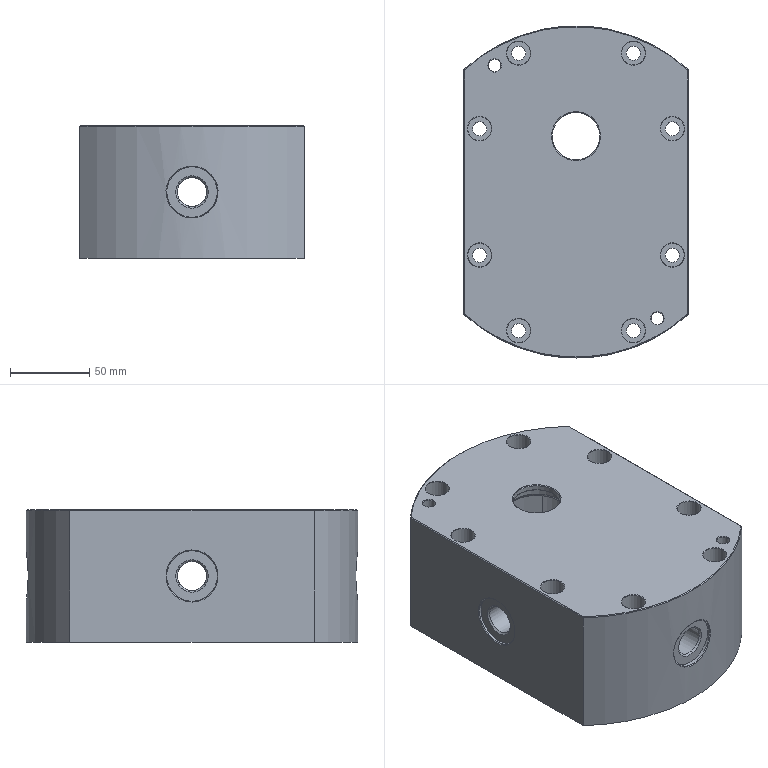NC program | NX | posted with a generic post | part box 142 x 210 x 84 mm
Whole program:
N10 G17 G21 G94 G90
(FLOOR_WALL , TOOL : D50)
N12 T02 M6
N14 G54
N16 G17 G0 G90 X46.563 Y-51.997 B0. C0. S1200 M3
N18 G43 Z30. H2
N20 Z2.65
N22 G94 G1 Z-0.35 F1000.
N24 X43.563
N26 X-43.563 F2000.
N28 Y-23.998
N30 X43.563
N32 Y4.001
N34 X-43.563
N36 Y32.
N38 X43.563
N40 X46.563
N42 Z2.65
N44 G0 Z30.
N46 X50.098 Y-51.997
N48 Z2.301
N50 G1 Z-0.699 F1000.
N52 X47.098
N54 X-47.098 F2000.
N56 Y-23.998
N58 X47.098
N60 Y4.001
N62 X-47.098
N64 Y32.
N66 X47.098
N68 X50.098
N70 Z2.301
N72 G0 Z30.
N74 X52.803 Y-51.997
N76 Z1.951
N78 G1 Z-1.049 F1000.
N80 X49.803
N82 X-49.803 F2000.
N84 Y-23.998
N86 X49.803
N88 Y4.001
N90 X-49.803
N92 Y32.
N94 X49.803
N96 X52.803
N98 Z1.951
N100 G0 Z30.
N102 X55.078 Y-51.997
N104 Z1.602
N106 G1 Z-1.398 F1000.
N108 X52.078
N110 X-52.078 F2000.
N112 Y-23.998
N114 X52.078
N116 Y4.001
N118 X-52.078
N120 Y32.
N122 X52.078
N124 X55.078
N126 Z1.602
N128 G0 Z30.
N130 X57.078 Y-51.997
N132 Z1.252
N134 G1 Z-1.748 F1000.
N136 X54.078
N138 X-54.078 F2000.
N140 Y-23.998
N142 X54.078
N144 Y4.001
N146 X-54.078
N148 Y32.
N150 X54.078
N152 X57.078
N154 Z1.252
N156 G0 Z30.
N158 X58.881 Y-51.997
N160 Z0.903
N162 G1 Z-2.097 F1000.
N164 X55.881
N166 X-55.881 F2000.
N168 Y-23.998
N170 X55.881
N172 Y4.001
N174 X-55.881
N176 Y32.
N178 X55.881
N180 X58.881
N182 Z0.903
N184 G0 Z30.
N186 X60.535 Y-51.997
N188 Z0.553
N190 G1 Z-2.447 F1000.
N192 X57.535
N194 X-57.535 F2000.
N196 Y-23.998
N198 X57.535
N200 Y4.001
N202 X-57.535
N204 Y32.
N206 X57.535
N208 X60.535
N210 Z0.553
N212 G0 Z30.
N214 X62.07 Y-51.997
N216 Z0.204
N218 G1 Z-2.796 F1000.
N220 X59.07
N222 X-59.07 F2000.
N224 Y-23.998
N226 X59.07
N228 Y4.001
N230 X-59.07
N232 Y32.
N234 X59.07
N236 X62.07
N238 Z0.204
N240 G0 Z30.
N242 X63.509 Y-51.997
N244 Z-0.146
N246 G1 Z-3.146 F1000.
N248 X60.509
N250 X-60.509 F2000.
N252 Y-23.998
N254 X60.509
N256 Y4.001
N258 X-60.509
N260 Y32.
N262 X60.509
N264 X63.509
N266 Z-0.146
N268 G0 Z30.
N270 X64.866 Y-51.997
N272 Z-0.495
N274 G1 Z-3.495 F1000.
N276 X61.866
N278 X-61.866 F2000.
N280 Y-23.998
N282 X61.866
N284 Y4.001
N286 X-61.866
N288 Y32.
N290 X61.866
N292 X64.866
N294 Z-0.495
N296 G0 Z30.
N298 X66.153 Y-51.997
N300 Z-0.845
N302 G1 Z-3.845 F1000.
N304 X63.153
N306 X-63.153 F2000.
N308 Y-23.998
N310 X63.153
N312 Y4.001
N314 X-63.153
N316 Y32.
N318 X63.153
N320 X66.153
N322 Z-0.845
N324 G0 Z30.
N326 X67.38 Y-51.997
N328 Z-1.194
N330 G1 Z-4.194 F1000.
N332 X64.38
N334 X-64.38 F2000.
N336 Y-23.998
N338 X64.38
N340 Y4.001
N342 X-64.38
N344 Y32.
N346 X64.38
N348 X67.38
N350 Z-1.194
N352 G0 Z30.
N354 X68.553 Y-51.997
N356 Z-1.544
N358 G1 Z-4.544 F1000.
N360 X65.553
N362 X-65.553 F2000.
N364 Y-23.998
N366 X65.553
N368 Y4.001
N370 X-65.553
N372 Y32.
N374 X65.553
N376 X68.553
N378 Z-1.544
N380 G0 Z30.
N382 X69.68 Y-51.997
N384 Z-1.893
N386 G1 Z-4.893 F1000.
N388 X66.68
N390 X-66.68 F2000.
N392 Y-23.998
N394 X66.68
N396 Y4.001
N398 X-66.68
N400 Y32.
N402 X66.68
N404 X69.68
N406 Z-1.893
N408 G0 Z30.
N410 X70.763 Y-51.997
N412 Z-2.243
N414 G1 Z-5.243 F1000.
N416 X67.763
N418 X-67.763 F2000.
N420 Y-23.998
N422 X67.763
N424 Y4.001
N426 X-67.763
N428 Y32.
N430 X67.763
N432 X70.763
N434 Z-2.243
N436 G0 Z30.
N438 X71.809 Y-51.997
N440 Z-2.592
N442 G1 Z-5.592 F1000.
N444 X68.809
N446 X-68.809 F2000.
N448 Y-23.998
N450 X68.809
N452 Y4.001
N454 X-68.809
N456 Y32.
N458 X68.809
N460 X71.809
N462 Z-2.592
N464 G0 Z30.
N466 X72.82 Y-51.997
N468 Z-2.941
N470 G1 Z-5.941 F1000.
N472 X69.82
N474 X-69.82 F2000.
N476 Y-23.998
N478 X69.82
N480 Y4.001
N482 X-69.82
N484 Y32.
N486 X69.82
N488 X72.82
N490 Z-2.941
N492 G0 Z30.
N494 X73.798 Y-51.997
N496 Z-3.291
N498 G1 Z-6.291 F1000.
N500 X70.798
N502 X-70.798 F2000.
N504 Y-23.998
N506 X70.798
N508 Y4.001
N510 X-70.798
N512 Y32.
N514 X70.798
N516 X73.798
N518 Z-3.291
N520 G0 Z30.
N522 X74.748 Y-51.997
N524 Z-3.64
N526 G1 Z-6.64 F1000.
N528 X71.748
N530 X-71.748 F2000.
N532 Y-23.998
N534 X71.748
N536 Y4.001
N538 X-71.748
N540 Y32.
N542 X71.748
N544 X74.748
N546 Z-3.64
N548 G0 Z30.
N550 X75.67 Y-51.997
N552 Z-3.99
N554 G1 Z-6.99 F1000.
N556 X72.67
N558 X-72.67 F2000.
N560 Y-23.998
N562 X72.67
N564 Y4.001
N566 X-72.67
N568 Y32.
N570 X72.67
N572 X75.67
N574 Z-3.99
N576 G0 Z30.
N578 X76.567 Y-51.997
N580 Z-4.339
N582 G1 Z-7.339 F1000.
N584 X73.567
N586 X-73.567 F2000.
N588 Y-23.998
N590 X73.567
N592 Y4.001
N594 X-73.567
N596 Y32.
N598 X73.567
N600 X76.567
N602 Z-4.339
N604 G0 Z30.
N606 X77.44 Y-51.997
N608 Z-4.689
N610 G1 Z-7.689 F1000.
N612 X74.44
N614 X-74.44 F2000.
N616 Y-23.998
N618 X74.44
N620 Y4.001
N622 X-74.44
N624 Y32.
N626 X74.44
N628 X77.44
N630 Z-4.689
N632 G0 Z30.
N634 X78.292 Y-51.997
N636 Z-5.038
N638 G1 Z-8.038 F1000.
N640 X75.292
N642 X-75.292 F2000.
N644 Y-23.998
N646 X75.292
N648 Y4.001
N650 X-75.292
N652 Y32.
N654 X75.292
N656 X78.292
N658 Z-5.038
N660 G0 Z30.
N662 X79.123 Y-51.997
N664 Z-5.388
N666 G1 Z-8.388 F1000.
N668 X76.123
N670 X-76.123 F2000.
N672 Y-23.998
N674 X76.123
N676 Y4.001
N678 X-76.123
N680 Y32.
N682 X76.123
N684 X79.123
N686 Z-5.388
N688 G0 Z30.
N690 X79.934 Y-51.997
N692 Z-5.737
N694 G1 Z-8.737 F1000.
N696 X76.934
N698 X-76.934 F2000.
N700 Y-23.998
N702 X76.934
N704 Y4.001
N706 X-76.934
N708 Y32.
N710 X76.934
N712 X79.934
N714 Z-5.737
N716 G0 Z30.
N718 X80.728 Y-51.997
N720 Z-6.087
N722 G1 Z-9.087 F1000.
N724 X77.728
N726 X-77.728 F2000.
N728 Y-23.998
N730 X77.728
N732 Y4.001
N734 X-77.728
N736 Y32.
N738 X77.728
N740 X80.728
N742 Z-6.087
N744 G0 Z30.
N746 X81.504 Y-51.997
N748 Z-6.436
N750 G1 Z-9.436 F1000.
N752 X78.504
N754 X-78.504 F2000.
N756 Y-23.998
N758 X78.504
N760 Y4.001
N762 X-78.504
N764 Y32.
N766 X78.504
N768 X81.504
N770 Z-6.436
N772 G0 Z30.
N774 X82.263 Y-51.997
N776 Z-6.786
N778 G1 Z-9.786 F1000.
N780 X79.263
N782 X-79.263 F2000.
N784 Y-23.998
N786 X79.263
N788 Y4.001
N790 X-79.263
N792 Y32.
N794 X79.263
N796 X82.263
N798 Z-6.786
N800 G0 Z30.
N802 X83.008 Y-51.997
N804 Z-7.135
N806 G1 Z-10.135 F1000.
N808 X80.008
N810 X-80.008 F2000.
N812 Y-23.998
N814 X80.008
N816 Y4.001
N818 X-80.008
N820 Y32.
N822 X80.008
N824 X83.008
N826 Z-7.135
N828 G0 Z30.
N830 X83.737 Y-51.997
N832 Z-7.485
N834 G1 Z-10.485 F1000.
N836 X80.737
N838 X-80.737 F2000.
N840 Y-23.998
N842 X80.737
N844 Y4.001
N846 X-80.737
N848 Y32.
N850 X80.737
N852 X83.737
N854 Z-7.485
N856 G0 Z30.
N858 X84.452 Y-51.997
N860 Z-7.834
N862 G1 Z-10.834 F1000.
N864 X81.452
N866 X-81.452 F2000.
N868 Y-23.998
N870 X81.452
N872 Y4.001
N874 X-81.452
N876 Y32.
N878 X81.452
N880 X84.452
N882 Z-7.834
N884 G0 Z30.
N886 X85.154 Y-51.997
N888 Z-8.184
N890 G1 Z-11.184 F1000.
N892 X82.154
N894 X-82.154 F2000.
N896 Y-23.998
N898 X82.154
N900 Y4.001
N902 X-82.154
N904 Y32.
N906 X82.154
N908 X85.154
N910 Z-8.184
N912 G0 Z30.
N914 X85.843 Y-51.997
N916 Z-8.533
N918 G1 Z-11.533 F1000.
N920 X82.843
N922 X-82.843 F2000.
N924 Y-23.998
N926 X82.843
N928 Y4.001
N930 X-82.843
N932 Y32.
N934 X82.843
N936 X85.843
N938 Z-8.533
N940 G0 Z30.
N942 X86.52 Y-51.997
N944 Z-8.883
N946 G1 Z-11.883 F1000.
N948 X83.52
N950 X-83.52 F2000.
N952 Y-23.998
N954 X83.52
N956 Y4.001
N958 X-83.52
N960 Y32.
N962 X83.52
N964 X86.52
N966 Z-8.883
N968 G0 Z30.
N970 X87.185 Y-51.997
N972 Z-9.232
N974 G1 Z-12.232 F1000.
N976 X84.185
N978 X-84.185 F2000.
N980 Y-23.998
N982 X84.185
N984 Y4.001
N986 X-84.185
N988 Y32.
N990 X84.185
N992 X87.185
N994 Z-9.232
N996 G0 Z30.
N998 X87.838 Y-51.997
N1000 Z-9.582
N1002 G1 Z-12.582 F1000.
N1004 X84.838
N1006 X-84.838 F2000.
N1008 Y-23.998
N1010 X84.838
N1012 Y4.001
N1014 X-84.838
N1016 Y32.
N1018 X84.838
N1020 X87.838
N1022 Z-9.582
N1024 G0 Z30.
N1026 X88.481 Y-51.997
N1028 Z-9.931
N1030 G1 Z-12.931 F1000.
N1032 X85.481
N1034 X-85.481 F2000.
N1036 Y-23.998
N1038 X85.481
N1040 Y4.001
N1042 X-85.481
N1044 Y32.
N1046 X85.481
N1048 X88.481
N1050 Z-9.931
N1052 G0 Z30.
N1054 X89.113 Y-51.997
N1056 Z-10.281
N1058 G1 Z-13.281 F1000.
N1060 X86.113
N1062 X-86.113 F2000.
N1064 Y-23.998
N1066 X86.113
N1068 Y4.001
N1070 X-86.113
N1072 Y32.
N1074 X86.113
N1076 X89.113
N1078 Z-10.281
N1080 G0 Z30.
N1082 X89.735 Y-51.997
N1084 Z-10.63
N1086 G1 Z-13.63 F1000.
N1088 X86.735
N1090 X-86.735 F2000.
N1092 Y-23.998
N1094 X86.735
N1096 Y4.001
N1098 X-86.735
N1100 Y32.
N1102 X86.735
N1104 X89.735
N1106 Z-10.63
N1108 G0 Z30.
N1110 X90.348 Y-51.997
N1112 Z-10.98
N1114 G1 Z-13.98 F1000.
N1116 X87.348
N1118 X-87.348 F2000.
N1120 Y-23.998
N1122 X87.348
N1124 Y4.001
N1126 X-87.348
N1128 Y32.
N1130 X87.348
N1132 X90.348
N1134 Z-10.98
N1136 G0 Z30.
N1138 X90.951 Y-51.997
N1140 Z-11.329
N1142 G1 Z-14.329 F1000.
N1144 X87.951
N1146 X-87.951 F2000.
N1148 Y-23.998
N1150 X87.951
N1152 Y4.001
N1154 X-87.951
N1156 Y32.
N1158 X87.951
N1160 X90.951
N1162 Z-11.329
N1164 G0 Z30.
N1166 X91.545 Y-51.997
N1168 Z-11.679
N1170 G1 Z-14.679 F1000.
N1172 X88.545
N1174 X-88.545 F2000.
N1176 Y-23.998
N1178 X88.545
N1180 Y4.001
N1182 X-88.545
N1184 Y32.
N1186 X88.545
N1188 X91.545
N1190 Z-11.679
N1192 G0 Z30.
N1194 X92.13 Y-51.997
N1196 Z-12.028
N1198 G1 Z-15.028 F1000.
N1200 X89.13
N1202 X-89.13 F2000.
N1204 Y-23.998
N1206 X89.13
N1208 Y4.001
N1210 X-89.13
N1212 Y32.
N1214 X89.13
N1216 X92.13
N1218 Z-12.028
N1220 G0 Z30.
N1222 X92.707 Y-51.997
N1224 Z-12.377
N1226 G1 Z-15.377 F1000.
N1228 X89.707
N1230 X-89.707 F2000.
N1232 Y-23.998
N1234 X89.707
N1236 Y4.001
N1238 X-89.707
N1240 Y32.
N1242 X89.707
N1244 X92.707
N1246 Z-12.377
N1248 G0 Z30.
N1250 X93.275 Y-51.997
N1252 Z-12.727
N1254 G1 Z-15.727 F1000.
N1256 X90.275
N1258 X-90.275 F2000.
N1260 Y-23.998
N1262 X90.275
N1264 Y4.001
N1266 X-90.275
N1268 Y32.
N1270 X90.275
N1272 X93.275
N1274 Z-12.727
N1276 G0 Z30.
N1278 X93.835 Y-51.997
N1280 Z-13.076
N1282 G1 Z-16.076 F1000.
N1284 X90.835
N1286 X-90.835 F2000.
N1288 Y-23.998
N1290 X90.835
N1292 Y4.001
N1294 X-90.835
N1296 Y32.
N1298 X90.835
N1300 X93.835
N1302 Z-13.076
N1304 G0 Z30.
N1306 X94.388 Y-51.997
N1308 Z-13.426
N1310 G1 Z-16.426 F1000.
N1312 X91.388
N1314 X-91.388 F2000.
N1316 Y-23.998
N1318 X91.388
N1320 Y4.001
N1322 X-91.388
N1324 Y32.
N1326 X91.388
N1328 X94.388
N1330 Z-13.426
N1332 G0 Z30.
N1334 X94.933 Y-51.997
N1336 Z-13.775
N1338 G1 Z-16.775 F1000.
N1340 X91.933
N1342 X-91.933 F2000.
N1344 Y-23.998
N1346 X91.933
N1348 Y4.001
N1350 X-91.933
N1352 Y32.
N1354 X91.933
N1356 X94.933
N1358 Z-13.775
N1360 G0 Z30.
N1362 X95.471 Y-51.997
N1364 Z-14.125
N1366 G1 Z-17.125 F1000.
N1368 X92.471
N1370 X-92.471 F2000.
N1372 Y-23.998
N1374 X92.471
N1376 Y4.001
N1378 X-92.471
N1380 Y32.
N1382 X92.471
N1384 X95.471
N1386 Z-14.125
N1388 G0 Z30.
N1390 X96.002 Y-51.997
N1392 Z-14.474
N1394 G1 Z-17.474 F1000.
N1396 X93.002
N1398 X-93.002 F2000.
N1400 Y-23.998
N1402 X93.002
N1404 Y4.001
N1406 X-93.002
N1408 Y32.
N1410 X93.002
N1412 X96.002
N1414 Z-14.474
N1416 G0 Z30.
N1418 X96.526 Y-51.997
N1420 Z-14.824
N1422 G1 Z-17.824 F1000.
N1424 X93.526
N1426 X-93.526 F2000.
N1428 Y-23.998
N1430 X93.526
N1432 Y4.001
N1434 X-93.526
N1436 Y32.
N1438 X93.526
N1440 X96.526
N1442 Z-14.824
N1444 G0 Z30.
N1446 X97.043 Y-51.997
N1448 Z-15.173
N1450 G1 Z-18.173 F1000.
N1452 X94.043
N1454 X-94.043 F2000.
N1456 Y-23.998
N1458 X94.043
N1460 Y4.001
N1462 X-94.043
N1464 Y32.
N1466 X94.043
N1468 X97.043
N1470 Z-15.173
N1472 G0 Z30.
N1474 X97.554 Y-51.997
N1476 Z-15.523
N1478 G1 Z-18.523 F1000.
N1480 X94.554
N1482 X-94.554 F2000.
N1484 Y-23.998
N1486 X94.554
N1488 Y4.001
N1490 X-94.554
N1492 Y32.
N1494 X94.554
N1496 X97.554
N1498 Z-15.523
N1500 G0 Z30.
N1502 X98.058 Y-51.997
N1504 Z-15.872
N1506 G1 Z-18.872 F1000.
N1508 X95.058
N1510 X-95.058 F2000.
N1512 Y-23.998
N1514 X95.058
N1516 Y4.001
N1518 X-95.058
N1520 Y32.
N1522 X95.058
N1524 X98.058
N1526 Z-15.872
N1528 G0 Z30.
N1530 X98.557 Y-51.997
N1532 Z-16.222
N1534 G1 Z-19.222 F1000.
N1536 X95.557
N1538 X-95.557 F2000.
N1540 Y-23.998
N1542 X95.557
N1544 Y4.001
N1546 X-95.557
N1548 Y32.
N1550 X95.557
N1552 X98.557
N1554 Z-16.222
N1556 G0 Z30.
N1558 X99.049 Y-51.997
N1560 Z-16.571
N1562 G1 Z-19.571 F1000.
N1564 X96.049
N1566 X-96.049 F2000.
N1568 Y-23.998
N1570 X96.049
N1572 Y4.001
N1574 X-96.049
N1576 Y32.
N1578 X96.049
N1580 X99.049
N1582 Z-16.571
N1584 G0 Z30.
N1586 X99.535 Y-51.997
N1588 Z-16.921
N1590 G1 Z-19.921 F1000.
N1592 X96.535
N1594 X-96.535 F2000.
N1596 Y-23.998
N1598 X96.535
N1600 Y4.001
N1602 X-96.535
N1604 Y32.
N1606 X96.535
N1608 X99.535
N1610 Z-16.921
N1612 G0 Z30.
N1614 X100.015 Y-51.997
N1616 Z-17.27
N1618 G1 Z-20.27 F1000.
N1620 X97.015
N1622 X-97.015 F2000.
N1624 Y-23.998
N1626 X97.015
N1628 Y4.001
N1630 X-97.015
N1632 Y32.
N1634 X97.015
N1636 X100.015
N1638 Z-17.27
N1640 G0 Z30.
N1642 X100.49 Y-51.997
N1644 Z-17.62
N1646 G1 Z-20.62 F1000.
N1648 X97.49
N1650 X-97.49 F2000.
N1652 Y-23.998
N1654 X97.49
N1656 Y4.001
N1658 X-97.49
N1660 Y32.
N1662 X97.49
N1664 X100.49
N1666 Z-17.62
N1668 G0 Z30.
N1670 X100.959 Y-51.997
N1672 Z-17.969
N1674 G1 Z-20.969 F1000.
N1676 X97.959
N1678 X-97.959 F2000.
N1680 Y-23.998
N1682 X97.959
N1684 Y4.001
N1686 X-97.959
N1688 Y32.
N1690 X97.959
N1692 X100.959
N1694 Z-17.969
N1696 G0 Z30.
N1698 X101.423 Y-51.997
N1700 Z-18.319
N1702 G1 Z-21.319 F1000.
N1704 X98.423
N1706 X-98.423 F2000.
N1708 Y-23.998
N1710 X98.423
N1712 Y4.001
N1714 X-98.423
N1716 Y32.
N1718 X98.423
N1720 X101.423
N1722 Z-18.319
N1724 G0 Z30.
N1726 X101.881 Y-51.997
N1728 Z-18.668
N1730 G1 Z-21.668 F1000.
N1732 X98.881
N1734 X-98.881 F2000.
N1736 Y-23.998
N1738 X98.881
N1740 Y4.001
N1742 X-98.881
N1744 Y32.
N1746 X98.881
N1748 X101.881
N1750 Z-18.668
N1752 G0 Z30.
N1754 X102.334 Y-51.997
N1756 Z-19.018
N1758 G1 Z-22.018 F1000.
N1760 X99.334
N1762 X-99.334 F2000.
N1764 Y-23.998
N1766 X99.334
N1768 Y4.001
N1770 X-99.334
N1772 Y32.
N1774 X99.334
N1776 X102.334
N1778 Z-19.018
N1780 G0 Z30.
N1782 X102.783 Y-51.997
N1784 Z-19.367
N1786 G1 Z-22.367 F1000.
N1788 X99.783
N1790 X-99.783 F2000.
N1792 Y-23.998
N1794 X99.783
N1796 Y4.001
N1798 X-99.783
N1800 Y32.
N1802 X99.783
N1804 X102.783
N1806 Z-19.367
N1808 G0 Z30.
N1810 X103.226 Y-51.997
N1812 Z-19.717
N1814 G1 Z-22.717 F1000.
N1816 X100.226
N1818 X-100.226 F2000.
N1820 Y-23.998
N1822 X100.226
N1824 Y4.001
N1826 X-100.226
N1828 Y32.
N1830 X100.226
N1832 X103.226
N1834 Z-19.717
N1836 G0 Z30.
N1838 X103.665 Y-51.997
N1840 Z-20.066
N1842 G1 Z-23.066 F1000.
N1844 X100.665
N1846 X-100.665 F2000.
N1848 Y-23.998
N1850 X100.665
N1852 Y4.001
N1854 X-100.665
N1856 Y32.
N1858 X100.665
N1860 X103.665
N1862 Z-20.066
N1864 G0 Z30.
N1866 X104.098 Y-51.997
N1868 Z-20.416
N1870 G1 Z-23.416 F1000.
N1872 X101.098
N1874 X-101.098 F2000.
N1876 Y-23.998
N1878 X101.098
N1880 Y4.001
N1882 X-101.098
N1884 Y32.
N1886 X101.098
N1888 X104.098
N1890 Z-20.416
N1892 G0 Z30.
N1894 X104.527 Y-51.997
N1896 Z-20.765
N1898 G1 Z-23.765 F1000.
N1900 X101.527
N1902 X-101.527 F2000.
N1904 Y-23.998
N1906 X101.527
N1908 Y4.001
N1910 X-101.527
N1912 Y32.
N1914 X101.527
N1916 X104.527
N1918 Z-20.765
N1920 G0 Z30.
N1922 X104.952 Y-51.997
N1924 Z-21.115
N1926 G1 Z-24.115 F1000.
N1928 X101.952
N1930 X-101.952 F2000.
N1932 Y-23.998
N1934 X101.952
N1936 Y4.001
N1938 X-101.952
N1940 Y32.
N1942 X101.952
N1944 X104.952
N1946 Z-21.115
N1948 G0 Z30.
N1950 X105.372 Y-51.997
N1952 Z-21.464
N1954 G1 Z-24.464 F1000.
N1956 X102.372
N1958 X-102.372 F2000.
N1960 Y-23.998
N1962 X102.372
N1964 Y4.001
N1966 X-102.372
N1968 Y32.
N1970 X102.372
N1972 X105.372
N1974 Z-21.464
N1976 G0 Z30.
N1978 X105.787 Y-51.997
N1980 Z-21.813
N1982 G1 Z-24.813 F1000.
N1984 X102.787
N1986 X-102.787 F2000.
N1988 Y-23.998
N1990 X102.787
N1992 Y4.001
N1994 X-102.787
N1996 Y32.
N1998 X102.787
N2000 X105.787
N2002 Z-21.813
N2004 G0 Z30.
N2006 X106.199 Y-51.997
N2008 Z-22.163
N2010 G1 Z-25.163 F1000.
N2012 X103.199
N2014 X-103.199 F2000.
N2016 Y-23.998
N2018 X103.199
N2020 Y4.001
N2022 X-103.199
N2024 Y32.
N2026 X103.199
N2028 X106.199
N2030 Z-22.163
N2032 G0 Z30.
N2034 X106.606 Y-51.997
N2036 Z-22.512
N2038 G1 Z-25.512 F1000.
N2040 X103.606
N2042 X-103.606 F2000.
N2044 Y-23.998
N2046 X103.606
N2048 Y4.001
N2050 X-103.606
N2052 Y32.
N2054 X103.606
N2056 X106.606
N2058 Z-22.512
N2060 G0 Z30.
N2062 X107.008 Y-51.997
N2064 Z-22.862
N2066 G1 Z-25.862 F1000.
N2068 X104.008
N2070 X-104.008 F2000.
N2072 Y-23.998
N2074 X104.008
N2076 Y4.001
N2078 X-104.008
N2080 Y32.
N2082 X104.008
N2084 X107.008
N2086 Z-22.862
N2088 G0 Z30.
N2090 X107.407 Y-51.997
N2092 Z-23.211
N2094 G1 Z-26.211 F1000.
N2096 X104.407
N2098 X-104.407 F2000.
N2100 Y-23.998
N2102 X104.407
N2104 Y4.001
N2106 X-104.407
N2108 Y32.
N2110 X104.407
N2112 X107.407
N2114 Z-23.211
N2116 G0 Z30.
N2118 X107.802 Y-51.997
N2120 Z-23.561
N2122 G1 Z-26.561 F1000.
N2124 X104.802
N2126 X-104.802 F2000.
N2128 Y-23.998
N2130 X104.802
N2132 Y4.001
N2134 X-104.802
N2136 Y32.
N2138 X104.802
N2140 X107.802
N2142 Z-23.561
N2144 G0 Z30.
N2146 X108.193 Y-51.997
N2148 Z-23.91
N2150 G1 Z-26.91 F1000.
N2152 X105.193
N2154 X-105.193 F2000.
N2156 Y-23.998
N2158 X105.193
N2160 Y4.001
N2162 X-105.193
N2164 Y32.
N2166 X105.193
N2168 X108.193
N2170 Z-23.91
N2172 G0 Z30.
N2174 X108.58 Y-51.997
N2176 Z-24.26
N2178 G1 Z-27.26 F1000.
N2180 X105.58
N2182 X-105.58 F2000.
N2184 Y-23.998
N2186 X105.58
N2188 Y4.001
N2190 X-105.58
N2192 Y32.
N2194 X105.58
N2196 X108.58
N2198 Z-24.26
N2200 G0 Z30.
N2202 X108.963 Y-51.997
N2204 Z-24.609
N2206 G1 Z-27.609 F1000.
N2208 X105.963
N2210 X-105.963 F2000.
N2212 Y-23.998
N2214 X105.963
N2216 Y4.001
N2218 X-105.963
N2220 Y32.
N2222 X105.963
N2224 X108.963
N2226 Z-24.609
N2228 G0 Z30.
N2230 X109.342 Y-51.997
N2232 Z-24.959
N2234 G1 Z-27.959 F1000.
N2236 X106.342
N2238 X-106.342 F2000.
N2240 Y-23.998
N2242 X106.342
N2244 Y4.001
N2246 X-106.342
N2248 Y32.
N2250 X106.342
N2252 X109.342
N2254 Z-24.959
N2256 G0 Z30.
N2258 X109.717 Y-51.997
N2260 Z-25.308
N2262 G1 Z-28.308 F1000.
N2264 X106.717
N2266 X-106.717 F2000.
N2268 Y-23.998
N2270 X106.717
N2272 Y4.001
N2274 X-106.717
N2276 Y32.
N2278 X106.717
N2280 X109.717
N2282 Z-25.308
N2284 G0 Z30.
N2286 X110.089 Y-51.997
N2288 Z-25.658
N2290 G1 Z-28.658 F1000.
N2292 X107.089
N2294 X-107.089 F2000.
N2296 Y-23.998
N2298 X107.089
N2300 Y4.001
N2302 X-107.089
N2304 Y32.
N2306 X107.089
N2308 X110.089
N2310 Z-25.658
N2312 G0 Z30.
N2314 X110.458 Y-51.997
N2316 Z-26.007
N2318 G1 Z-29.007 F1000.
N2320 X107.458
N2322 X-107.458 F2000.
N2324 Y-23.998
N2326 X107.458
N2328 Y4.001
N2330 X-107.458
N2332 Y32.
N2334 X107.458
N2336 X110.458
N2338 Z-26.007
N2340 G0 Z30.
N2342 X110.822 Y-51.997
N2344 Z-26.357
N2346 G1 Z-29.357 F1000.
N2348 X107.822
N2350 X-107.822 F2000.
N2352 Y-23.998
N2354 X107.822
N2356 Y4.001
N2358 X-107.822
N2360 Y32.
N2362 X107.822
N2364 X110.822
N2366 Z-26.357
N2368 G0 Z30.
N2370 X111.184 Y-51.997
N2372 Z-26.706
N2374 G1 Z-29.706 F1000.
N2376 X108.184
N2378 X-108.184 F2000.
N2380 Y-23.998
N2382 X108.184
N2384 Y4.001
N2386 X-108.184
N2388 Y32.
N2390 X108.184
N2392 X111.184
N2394 Z-26.706
N2396 G0 Z30.
N2398 X111.542 Y-51.997
N2400 Z-27.056
N2402 G1 Z-30.056 F1000.
N2404 X108.542
N2406 X-108.542 F2000.
N2408 Y-23.998
N2410 X108.542
N2412 Y4.001
N2414 X-108.542
N2416 Y32.
N2418 X108.542
N2420 X111.542
N2422 Z-27.056
N2424 G0 Z30.
N2426 X111.896 Y-51.997
N2428 Z-27.405
N2430 G1 Z-30.405 F1000.
N2432 X108.896
N2434 X-108.896 F2000.
N2436 Y-23.998
N2438 X108.896
N2440 Y4.001
N2442 X-108.896
N2444 Y32.
N2446 X108.896
N2448 X111.896
N2450 Z-27.405
N2452 G0 Z30.
N2454 X112.247 Y-51.997
N2456 Z-27.755
N2458 G1 Z-30.755 F1000.
N2460 X109.247
N2462 X-109.247 F2000.
N2464 Y-23.998
N2466 X109.247
N2468 Y4.001
N2470 X-109.247
N2472 Y32.
N2474 X109.247
N2476 X112.247
N2478 Z-27.755
N2480 G0 Z30.
N2482 X112.595 Y-51.997
N2484 Z-28.104
N2486 G1 Z-31.104 F1000.
N2488 X109.595
N2490 X-109.595 F2000.
N2492 Y-23.998
N2494 X109.595
N2496 Y4.001
N2498 X-109.595
N2500 Y32.
N2502 X109.595
N2504 X112.595
N2506 Z-28.104
N2508 G0 Z30.
N2510 X112.94 Y-51.997
N2512 Z-28.454
N2514 G1 Z-31.454 F1000.
N2516 X109.94
N2518 X-109.94 F2000.
N2520 Y-23.998
N2522 X109.94
N2524 Y4.001
N2526 X-109.94
N2528 Y32.
N2530 X109.94
N2532 X112.94
N2534 Z-28.454
N2536 G0 Z30.
N2538 X113.281 Y-51.997
N2540 Z-28.803
N2542 G1 Z-31.803 F1000.
N2544 X110.281
N2546 X-110.281 F2000.
N2548 Y-23.998
N2550 X110.281
N2552 Y4.001
N2554 X-110.281
N2556 Y32.
N2558 X110.281
N2560 X113.281
N2562 Z-28.803
N2564 G0 Z30.
N2566 X113.619 Y-51.997
N2568 Z-29.153
N2570 G1 Z-32.153 F1000.
N2572 X110.619
N2574 X-110.619 F2000.
N2576 Y-23.998
N2578 X110.619
N2580 Y4.001
N2582 X-110.619
N2584 Y32.
N2586 X110.619
N2588 X113.619
N2590 Z-29.153
N2592 G0 Z30.
N2594 X113.954 Y-51.997
N2596 Z-29.502
N2598 G1 Z-32.502 F1000.
N2600 X110.954
N2602 X-110.954 F2000.
N2604 Y-23.998
N2606 X110.954
N2608 Y4.001
N2610 X-110.954
N2612 Y32.
N2614 X110.954
N2616 X113.954
N2618 Z-29.502
N2620 G0 Z30.
N2622 X114.286 Y-51.997
N2624 Z-29.852
N2626 G1 Z-32.852 F1000.
N2628 X111.286
N2630 X-111.286 F2000.
N2632 Y-23.998
N2634 X111.286
N2636 Y4.001
N2638 X-111.286
N2640 Y32.
N2642 X111.286
N2644 X114.286
N2646 Z-29.852
N2648 G0 Z30.
N2650 X114.615 Y-51.997
N2652 Z-30.201
N2654 G1 Z-33.201 F1000.
N2656 X111.615
N2658 X-111.615 F2000.
N2660 Y-23.998
N2662 X111.615
N2664 Y4.001
N2666 X-111.615
N2668 Y32.
N2670 X111.615
N2672 X114.615
N2674 Z-30.201
N2676 G0 Z30.
N2678 X114.941 Y-51.997
N2680 Z-30.551
N2682 G1 Z-33.551 F1000.
N2684 X111.941
N2686 X-111.941 F2000.
N2688 Y-23.998
N2690 X111.941
N2692 Y4.001
N2694 X-111.941
N2696 Y32.
N2698 X111.941
N2700 X114.941
N2702 Z-30.551
N2704 G0 Z30.
N2706 X115.264 Y-51.997
N2708 Z-30.9
N2710 G1 Z-33.9 F1000.
N2712 X112.264
N2714 X-112.264 F2000.
N2716 Y-23.998
N2718 X112.264
N2720 Y4.001
N2722 X-112.264
N2724 Y32.
N2726 X112.264
N2728 X115.264
N2730 Z-30.9
N2732 G0 Z30.
(FLOOR_WALL_COPY , TOOL : D50)
N2734 X115.356 Y-51.997 S2500
N2736 Z-31.
N2738 G1 Z-34. F1000.
N2740 X112.356
N2742 X-112.356
N2744 Y-23.998
N2746 X112.356
N2748 Y4.001
N2750 X-112.356
N2752 Y32.
N2754 X112.356
N2756 X115.356
N2758 Z-31.
N2760 G0 Z30.
N2762 M5
(HOLE_MILLING , TOOL : D10)
N2764 T10 M6
N2766 G54
N2768 G17 G0 G90 X0. Y0. B0. C0. S3000 M3
N2770 G43 Z30. H10
N2772 Z-33.5
N2774 G94 G3 X-1.817 Y1.817 R1.817 F2200.
N2776 X-3.633 Y0. R1.817
N2778 X-3.633 Y0. Z-33.72 I3.633 J0.
N2780 X-3.633 Y0. Z-33.94 I3.633 J0.
N2782 X-3.633 Y0. Z-34.16 I3.633 J0.
N2784 X-3.633 Y0. Z-34.38 I3.633 J0.
N2786 X-3.633 Y0. Z-34.6 I3.633 J0.
N2788 X-3.633 Y0. Z-34.82 I3.633 J0.
N2790 X-3.633 Y0. Z-35.04 I3.633 J0.
N2792 X-3.633 Y0. Z-35.26 I3.633 J0.
N2794 X-3.633 Y0. Z-35.48 I3.633 J0.
N2796 X-3.633 Y0. Z-35.7 I3.633 J0.
N2798 X-3.633 Y0. Z-35.92 I3.633 J0.
N2800 X2.379 Y-2.746 Z-36. R3.633
N2802 X2.746 Y2.379 R3.633
N2804 X2.379 Y-2.746 R-3.633
N2806 X2.563 Y-0.183 R1.817
N2808 X0. Y0. R1.817
N2810 G0 Z-33.5
N2812 G3 X-3.633 Y3.633 R3.633
N2814 X-7.267 Y0. R3.633
N2816 X-7.267 Y0. Z-33.72 I7.267 J0.
N2818 X-7.267 Y0. Z-33.94 I7.267 J0.
N2820 X-7.267 Y0. Z-34.16 I7.267 J0.
N2822 X-7.267 Y0. Z-34.38 I7.267 J0.
N2824 X-7.267 Y0. Z-34.6 I7.267 J0.
N2826 X-7.267 Y0. Z-34.82 I7.267 J0.
N2828 X-7.267 Y0. Z-35.04 I7.267 J0.
N2830 X-7.267 Y0. Z-35.26 I7.267 J0.
N2832 X-7.267 Y0. Z-35.48 I7.267 J0.
N2834 X-7.267 Y0. Z-35.7 I7.267 J0.
N2836 X-7.267 Y0. Z-35.92 I7.267 J0.
N2838 X4.759 Y-5.492 Z-36. R7.267
N2840 X5.492 Y4.759 R7.267
N2842 X4.759 Y-5.492 R-7.267
N2844 X5.125 Y-0.367 R3.633
N2846 X0. Y0. R3.633
N2848 G0 Z-33.5
N2850 G3 X-5.45 Y5.45 R5.45
N2852 X-10.9 Y0. R5.45
N2854 X-10.9 Y0. Z-33.72 I10.9 J0.
N2856 X-10.9 Y0. Z-33.94 I10.9 J0.
N2858 X-10.9 Y0. Z-34.16 I10.9 J0.
N2860 X-10.9 Y0. Z-34.38 I10.9 J0.
N2862 X-10.9 Y0. Z-34.6 I10.9 J0.
N2864 X-10.9 Y0. Z-34.82 I10.9 J0.
N2866 X-10.9 Y0. Z-35.04 I10.9 J0.
N2868 X-10.9 Y0. Z-35.26 I10.9 J0.
N2870 X-10.9 Y0. Z-35.48 I10.9 J0.
N2872 X-10.9 Y0. Z-35.7 I10.9 J0.
N2874 X-10.9 Y0. Z-35.92 I10.9 J0.
N2876 X7.138 Y-8.238 Z-36. R10.9
N2878 X8.238 Y7.138 R10.9
N2880 X7.138 Y-8.238 R-10.9
N2882 X7.688 Y-0.55 R5.45
N2884 X0. Y0. R5.45
N2886 G0 Z30.
(HOLE_MILLING_COPY , TOOL : D10)
N2888 Z-35.5
N2890 G3 X-2.075 Y2.075 R2.075
N2892 X-4.15 Y0. R2.075
N2894 X-4.15 Y0. Z-35.72 I4.15 J0.
N2896 X-4.15 Y0. Z-35.94 I4.15 J0.
N2898 X-4.15 Y0. Z-36.16 I4.15 J0.
N2900 X-4.15 Y0. Z-36.38 I4.15 J0.
N2902 X-4.15 Y0. Z-36.6 I4.15 J0.
N2904 X-4.15 Y0. Z-36.82 I4.15 J0.
N2906 X-4.15 Y0. Z-37.04 I4.15 J0.
N2908 X-4.15 Y0. Z-37.26 I4.15 J0.
N2910 X-4.15 Y0. Z-37.48 I4.15 J0.
N2912 X-4.15 Y0. Z-37.7 I4.15 J0.
N2914 X-4.15 Y0. Z-37.92 I4.15 J0.
N2916 X-4.15 Y0. Z-38.14 I4.15 J0.
N2918 X-4.15 Y0. Z-38.36 I4.15 J0.
N2920 X-4.15 Y0. Z-38.58 I4.15 J0.
N2922 X-4.15 Y0. Z-38.8 I4.15 J0.
N2924 X-4.15 Y0. Z-39.02 I4.15 J0.
N2926 X-4.15 Y0. Z-39.24 I4.15 J0.
N2928 X-4.15 Y0. Z-39.46 I4.15 J0.
N2930 X-4.15 Y0. Z-39.68 I4.15 J0.
N2932 X-4.15 Y0. Z-39.9 I4.15 J0.
N2934 X-4.15 Y0. Z-40.12 I4.15 J0.
N2936 X-4.15 Y0. Z-40.34 I4.15 J0.
N2938 X-4.15 Y0. Z-40.56 I4.15 J0.
N2940 X-4.15 Y0. Z-40.78 I4.15 J0.
N2942 X-4.15 Y0. Z-41. I4.15 J0.
N2944 X-4.15 Y0. Z-41.22 I4.15 J0.
N2946 X-4.15 Y0. Z-41.44 I4.15 J0.
N2948 X-4.15 Y0. Z-41.66 I4.15 J0.
N2950 X-4.15 Y0. Z-41.88 I4.15 J0.
N2952 X-4.15 Y0. Z-42.1 I4.15 J0.
N2954 X-4.15 Y0. Z-42.32 I4.15 J0.
N2956 X-4.15 Y0. Z-42.54 I4.15 J0.
N2958 X-4.15 Y0. Z-42.76 I4.15 J0.
N2960 X-4.15 Y0. Z-42.98 I4.15 J0.
N2962 X-4.15 Y0. Z-43.2 I4.15 J0.
N2964 X-4.15 Y0. Z-43.42 I4.15 J0.
N2966 X-4.15 Y0. Z-43.64 I4.15 J0.
N2968 X-4.15 Y0. Z-43.86 I4.15 J0.
N2970 X-4.15 Y0. Z-44.08 I4.15 J0.
N2972 X-4.15 Y0. Z-44.3 I4.15 J0.
N2974 X-4.15 Y0. Z-44.52 I4.15 J0.
N2976 X-4.15 Y0. Z-44.74 I4.15 J0.
N2978 X-4.15 Y0. Z-44.96 I4.15 J0.
N2980 X-4.15 Y0. Z-45.18 I4.15 J0.
N2982 X-4.15 Y0. Z-45.4 I4.15 J0.
N2984 X-4.15 Y0. Z-45.62 I4.15 J0.
N2986 X-4.15 Y0. Z-45.84 I4.15 J0.
N2988 X-4.15 Y0. Z-46.06 I4.15 J0.
N2990 X-4.15 Y0. Z-46.28 I4.15 J0.
N2992 X-4.15 Y0. Z-46.5 I4.15 J0.
N2994 X-4.15 Y0. Z-46.72 I4.15 J0.
N2996 X-4.15 Y0. Z-46.94 I4.15 J0.
N2998 X-4.15 Y0. Z-47.16 I4.15 J0.
N3000 X-4.15 Y0. Z-47.38 I4.15 J0.
N3002 X-4.15 Y0. Z-47.6 I4.15 J0.
N3004 X-4.15 Y0. Z-47.82 I4.15 J0.
N3006 X-4.15 Y0. Z-48.04 I4.15 J0.
N3008 X-4.15 Y0. Z-48.26 I4.15 J0.
N3010 X-4.15 Y0. Z-48.48 I4.15 J0.
N3012 X-4.15 Y0. Z-48.7 I4.15 J0.
N3014 X-4.15 Y0. Z-48.92 I4.15 J0.
N3016 X-4.15 Y0. Z-49.14 I4.15 J0.
N3018 X-4.15 Y0. Z-49.36 I4.15 J0.
N3020 X-4.15 Y0. Z-49.58 I4.15 J0.
N3022 X-4.15 Y0. Z-49.8 I4.15 J0.
N3024 X-4.15 Y0. Z-50.02 I4.15 J0.
N3026 X-4.15 Y0. Z-50.24 I4.15 J0.
N3028 X-4.15 Y0. Z-50.46 I4.15 J0.
N3030 X-4.15 Y0. Z-50.68 I4.15 J0.
N3032 X-4.15 Y0. Z-50.9 I4.15 J0.
N3034 X-4.15 Y0. Z-51.12 I4.15 J0.
N3036 X-4.15 Y0. Z-51.34 I4.15 J0.
N3038 X-4.15 Y0. Z-51.56 I4.15 J0.
N3040 X-4.15 Y0. Z-51.78 I4.15 J0.
N3042 X-4.15 Y0. Z-52. I4.15 J0.
N3044 X-4.15 Y0. Z-52.22 I4.15 J0.
N3046 X-4.15 Y0. Z-52.44 I4.15 J0.
N3048 X-4.15 Y0. Z-52.66 I4.15 J0.
N3050 X-4.15 Y0. Z-52.88 I4.15 J0.
N3052 X-4.15 Y0. Z-53.1 I4.15 J0.
N3054 X-4.15 Y0. Z-53.32 I4.15 J0.
N3056 X-4.15 Y0. Z-53.54 I4.15 J0.
N3058 X-4.15 Y0. Z-53.76 I4.15 J0.
N3060 X-4.15 Y0. Z-53.98 I4.15 J0.
N3062 X-4.15 Y0. Z-54.2 I4.15 J0.
N3064 X-4.15 Y0. Z-54.42 I4.15 J0.
N3066 X-4.15 Y0. Z-54.64 I4.15 J0.
N3068 X-4.15 Y0. Z-54.86 I4.15 J0.
N3070 X-4.15 Y0. Z-55.08 I4.15 J0.
N3072 X-4.15 Y0. Z-55.3 I4.15 J0.
N3074 X-4.15 Y0. Z-55.52 I4.15 J0.
N3076 X-4.15 Y0. Z-55.74 I4.15 J0.
N3078 X-4.15 Y0. Z-55.96 I4.15 J0.
N3080 X-4.15 Y0. Z-56.18 I4.15 J0.
N3082 X-4.15 Y0. Z-56.4 I4.15 J0.
N3084 X-4.15 Y0. Z-56.62 I4.15 J0.
N3086 X-4.15 Y0. Z-56.84 I4.15 J0.
N3088 X-4.15 Y0. Z-57.06 I4.15 J0.
N3090 X-4.15 Y0. Z-57.28 I4.15 J0.
N3092 X-4.15 Y0. Z-57.5 I4.15 J0.
N3094 X-4.15 Y0. Z-57.72 I4.15 J0.
N3096 X-4.15 Y0. Z-57.94 I4.15 J0.
N3098 X-4.15 Y0. Z-58.16 I4.15 J0.
N3100 X-4.15 Y0. Z-58.38 I4.15 J0.
N3102 X-4.15 Y0. Z-58.6 I4.15 J0.
N3104 X-4.15 Y0. Z-58.82 I4.15 J0.
N3106 X-4.15 Y0. Z-59.04 I4.15 J0.
N3108 X-4.15 Y0. Z-59.26 I4.15 J0.
N3110 X-4.15 Y0. Z-59.48 I4.15 J0.
N3112 X-4.15 Y0. Z-59.7 I4.15 J0.
N3114 X-4.15 Y0. Z-59.92 I4.15 J0.
N3116 X2.718 Y-3.136 Z-60. R4.15
N3118 X3.136 Y2.718 R4.15
N3120 X2.718 Y-3.136 R-4.15
N3122 X2.927 Y-0.209 R2.075
N3124 X0. Y0. R2.075
N3126 G0 Z30.
N3128 M5
(HOLE_MILLING_COPY_1 , TOOL : D10JING)
N3130 T11 M6
N3132 G54
N3134 G17 G0 G90 X0. Y0. B0. C0. S5000 M3
N3136 G43 Z30. H11
N3138 Z-36.
N3140 G94 G1 X-7.486 Y2.524 F1000.
N3142 G3 X-11. Y0. R2.663
N3144 X0. Y-11. R11.
N3146 X-11. Y0. R-11.
N3148 X-7.486 Y-2.524 R2.663
N3150 G1 X0. Y0.
N3152 G0 Z30.
(HOLE_MILLING_COPY_1_COPY , TOOL : D10JING)
N3154 Z-58.
N3156 G3 X-2.125 Y2.125 R2.125
N3158 X-4.25 Y0. R2.125
N3160 X0. Y-4.25 R4.25
N3162 X-4.25 Y0. R-4.25
N3164 X-2.125 Y-2.125 R2.125
N3166 X0. Y0. R2.125
N3168 G0 Z30.
N3170 M5
(PLANAR_MILL , TOOL : D6A45)
N3172 T07 M6
N3174 G54
N3176 G17 G0 G90 X-1.543 Y-14.216 B0. C0. S7500 M3
N3178 G43 Z30. H7
N3180 Z-32.
N3182 G94 G1 Z-35. F1250.
N3184 X-0.766 Y-15.143
N3186 G3 X0. Y-15.5 R1.
N3188 X15.5 Y0. R15.5
N3190 X0. Y-15.5 R-15.5
N3192 X0.766 Y-15.143 R1.
N3194 G1 X1.543 Y-14.216
N3196 Z-32.
N3198 G0 Z30.
N3200 X-78.83 Y43.2
N3202 Z-32.
N3204 G1 Z-35.
N3206 X-78.122 Y42.357
N3208 G3 X-77.356 Y42. R1.
N3210 G1 X77.356
N3212 G3 X78.122 Y42.357 R1.
N3214 G1 X78.83 Y43.2
N3216 Z-32.
N3218 G0 Z30.
N3220 Y-43.7
N3222 Z-32.
N3224 G1 Z-35.
N3226 X78.122 Y-42.857
N3228 G3 X77.356 Y-42.5 R1.
N3230 G1 X-77.356
N3232 G3 X-78.122 Y-42.857 R1.
N3234 G1 X-78.83 Y-43.7
N3236 Z-32.
N3238 G0 Z30.
(PLANAR_MILL_COPY , TOOL : D6A45)
N3240 X-1.634 Y-6.858
N3242 Z-34.5
N3244 G1 Z-37.5
N3246 X-0.766 Y-7.893
N3248 G3 X0. Y-8.25 R1.
N3250 X8.25 Y0. R8.25
N3252 X0. Y-8.25 R-8.25
N3254 X0.766 Y-7.893 R1.
N3256 G1 X1.634 Y-6.858
N3258 Z-34.5
N3260 G0 Z30.
N3262 M5
N3264 M2